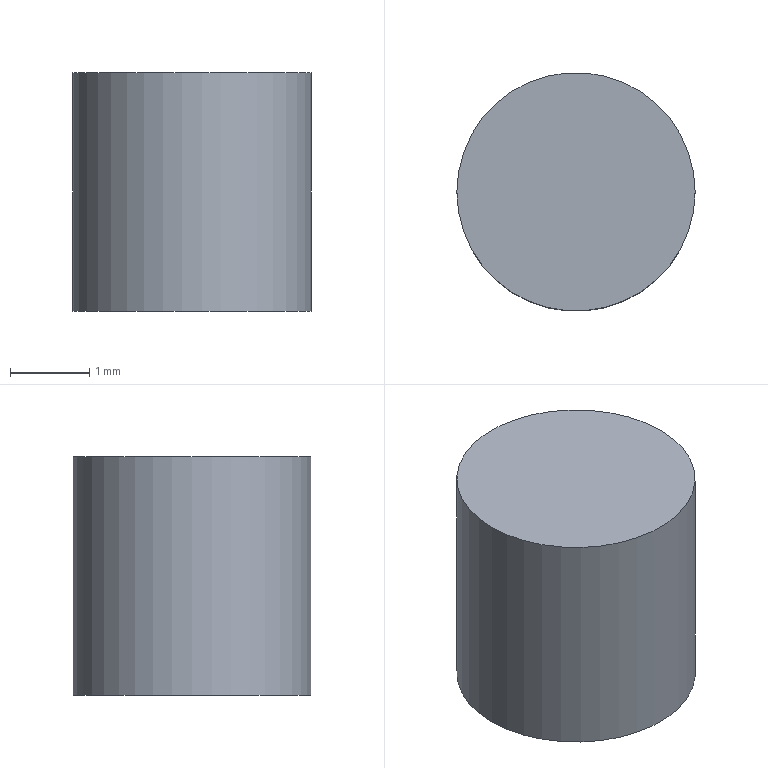Part | NX | features CYLINDER 1, DATUM_CSYS 1 | 1 solid | 3 faces | box 3 x 3 x 3 mm | volume 21.206 mm3 | plane 2 | cylinder 1 | commonest cylinder face diameters 3 x1
STEP:
#1=CARTESIAN_POINT('',(1.5,0.,3.));
#2=VERTEX_POINT('',#1);
#3=CARTESIAN_POINT('',(0.,0.,3.));
#4=DIRECTION('',(0.,0.,-1.));
#5=DIRECTION('',(1.,0.,0.));
#6=AXIS2_PLACEMENT_3D('',#3,#4,#5);
#7=CIRCLE('',#6,1.5);
#8=EDGE_CURVE('',#2,#2,#7,.T.);
#9=ORIENTED_EDGE('',*,*,#8,.F.);
#10=EDGE_LOOP('',(#9));
#11=FACE_BOUND('',#10,.T.);
#12=CARTESIAN_POINT('',(0.,0.,3.));
#13=DIRECTION('',(0.,0.,1.));
#14=DIRECTION('',(1.,0.,0.));
#15=AXIS2_PLACEMENT_3D('',#12,#13,#14);
#16=PLANE('',#15);
#17=ADVANCED_FACE('',(#11),#16,.T.);
#18=CARTESIAN_POINT('',(1.5,0.,0.));
#19=VERTEX_POINT('',#18);
#20=CARTESIAN_POINT('',(0.,0.,0.));
#21=DIRECTION('',(0.,0.,1.));
#22=DIRECTION('',(1.,0.,0.));
#23=AXIS2_PLACEMENT_3D('',#20,#21,#22);
#24=CIRCLE('',#23,1.5);
#25=EDGE_CURVE('',#19,#19,#24,.T.);
#26=ORIENTED_EDGE('',*,*,#25,.F.);
#27=EDGE_LOOP('',(#26));
#28=FACE_BOUND('',#27,.T.);
#29=CARTESIAN_POINT('',(0.,0.,0.));
#30=DIRECTION('',(0.,0.,-1.));
#31=DIRECTION('',(-1.,0.,0.));
#32=AXIS2_PLACEMENT_3D('',#29,#30,#31);
#33=PLANE('',#32);
#34=ADVANCED_FACE('',(#28),#33,.T.);
#35=ORIENTED_EDGE('',*,*,#8,.T.);
#36=EDGE_LOOP('',(#35));
#37=FACE_BOUND('',#36,.T.);
#38=ORIENTED_EDGE('',*,*,#25,.T.);
#39=EDGE_LOOP('',(#38));
#40=FACE_BOUND('',#39,.T.);
#41=CARTESIAN_POINT('',(0.,0.,0.));
#42=DIRECTION('',(0.,0.,1.));
#43=DIRECTION('',(1.,0.,0.));
#44=AXIS2_PLACEMENT_3D('',#41,#42,#43);
#45=CYLINDRICAL_SURFACE('',#44,1.5);
#46=ADVANCED_FACE('',(#37,#40),#45,.T.);
#47=CLOSED_SHELL('',(#17,#34,#46));
#48=MANIFOLD_SOLID_BREP('',#47);
#49=(LENGTH_UNIT()NAMED_UNIT(*)SI_UNIT(.MILLI.,.METRE.));
#50=UNCERTAINTY_MEASURE_WITH_UNIT(LENGTH_MEASURE(0.00001),#49,'','');
#51=(NAMED_UNIT(*)PLANE_ANGLE_UNIT()SI_UNIT($,.RADIAN.));
#52=(NAMED_UNIT(*)SI_UNIT($,.STERADIAN.)SOLID_ANGLE_UNIT());
#53=(GEOMETRIC_REPRESENTATION_CONTEXT(3)GLOBAL_UNCERTAINTY_ASSIGNED_CONTEXT((#50))GLOBAL_UNIT_ASSIGNED_CONTEXT((#49,#51,#52))REPRESENTATION_CONTEXT('',''));
#54=ADVANCED_BREP_SHAPE_REPRESENTATION('',(#48),#53);